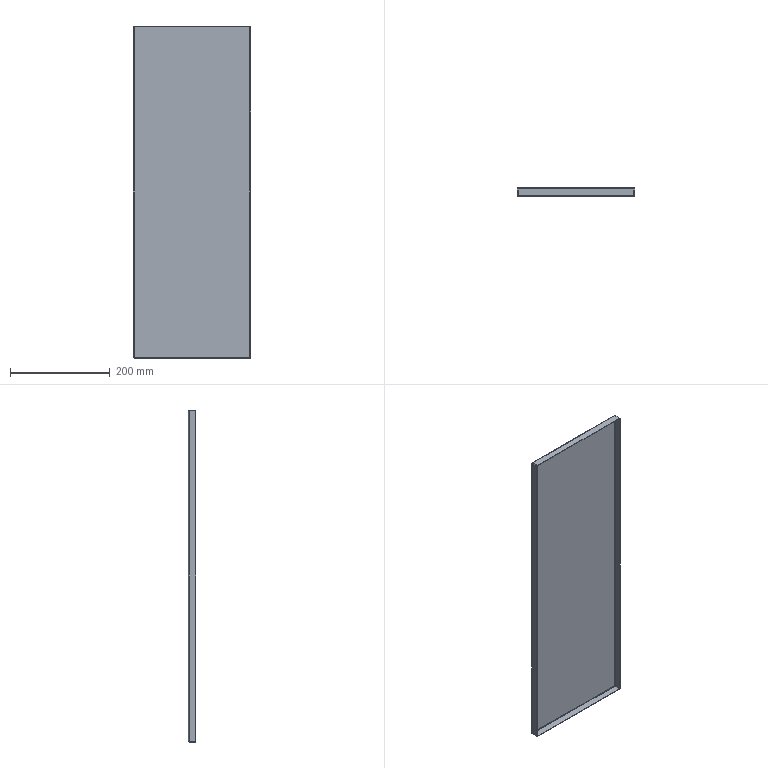Part | SolidWorks | features BaseBody 1 | 1 solid | 38 faces | box 236 x 15 x 666 mm | volume 181090 mm3 | plane 22 | cylinder 8 | spline 8 | commonest cylinder face diameters 2 x4 4 x4